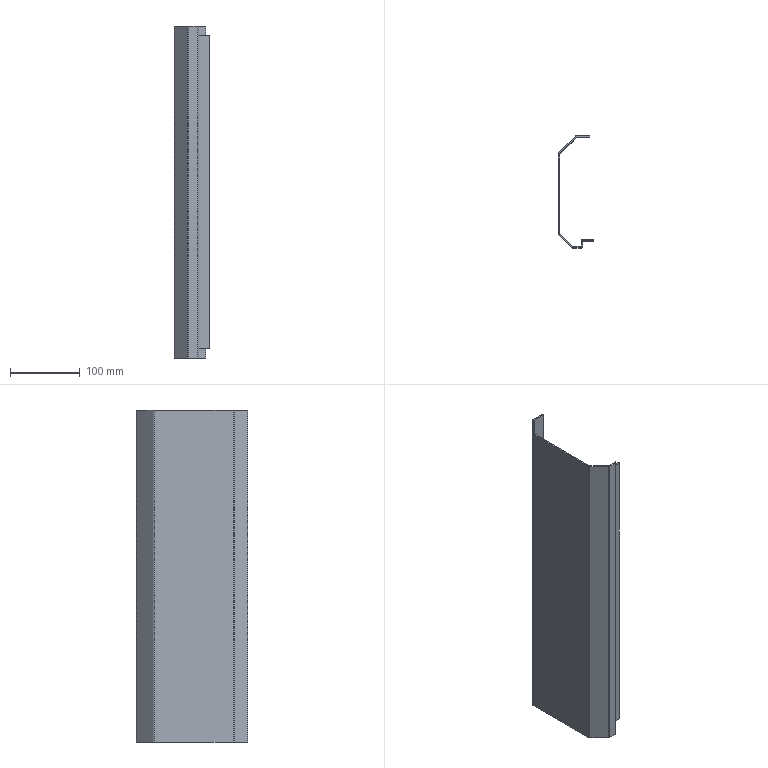Part | STEP file | Control Box 1 | 1 solid | 34 faces | box 51 x 160 x 476 mm | volume 222530 mm3 | plane 22 | cylinder 12 | commonest cylinder face diameters 0.2 x6 4.2 x6
STEP:
#1=CARTESIAN_POINT('',(-54.818,-25.87,476.));
#2=VERTEX_POINT('',#1);
#3=CARTESIAN_POINT('',(-54.818,-139.13,476.));
#4=VERTEX_POINT('',#3);
#5=CARTESIAN_POINT('',(-54.818,-25.,476.));
#6=DIRECTION('',(0.,-1.,0.));
#7=VECTOR('',#6,1000.);
#8=LINE('',#5,#7);
#9=EDGE_CURVE('',#2,#4,#8,.T.);
#10=ORIENTED_EDGE('',*,*,#9,.T.);
#11=CARTESIAN_POINT('',(-54.818,-139.13,0.));
#12=VERTEX_POINT('',#11);
#13=CARTESIAN_POINT('',(-54.818,-139.13,476.));
#14=DIRECTION('',(0.,0.,-1.));
#15=VECTOR('',#14,1000.);
#16=LINE('',#13,#15);
#17=EDGE_CURVE('',#4,#12,#16,.T.);
#18=ORIENTED_EDGE('',*,*,#17,.T.);
#19=CARTESIAN_POINT('',(-54.818,-25.87,0.));
#20=VERTEX_POINT('',#19);
#21=CARTESIAN_POINT('',(-54.818,-25.,0.));
#22=DIRECTION('',(0.,1.,0.));
#23=VECTOR('',#22,1000.);
#24=LINE('',#21,#23);
#25=EDGE_CURVE('',#12,#20,#24,.T.);
#26=ORIENTED_EDGE('',*,*,#25,.T.);
#27=CARTESIAN_POINT('',(-54.818,-25.87,476.));
#28=DIRECTION('',(0.,0.,1.));
#29=VECTOR('',#28,1000.);
#30=LINE('',#27,#29);
#31=EDGE_CURVE('',#20,#2,#30,.T.);
#32=ORIENTED_EDGE('',*,*,#31,.T.);
#33=EDGE_LOOP('',(#10,#18,#26,#32));
#34=FACE_OUTER_BOUND('',#33,.T.);
#35=CARTESIAN_POINT('',(-54.818,-25.,476.));
#36=DIRECTION('',(1.,0.,0.));
#37=DIRECTION('',(0.,1.,0.));
#38=AXIS2_PLACEMENT_3D('',#35,#36,#37);
#39=PLANE('',#38);
#40=ADVANCED_FACE('',(#34),#39,.T.);
#41=ORIENTED_EDGE('',*,*,#17,.F.);
#42=CARTESIAN_POINT('',(-54.789,-139.201,476.));
#43=VERTEX_POINT('',#42);
#44=CARTESIAN_POINT('',(-54.718,-139.13,476.));
#45=DIRECTION('',(0.,0.,-1.));
#46=DIRECTION('',(-1.,0.,0.));
#47=AXIS2_PLACEMENT_3D('',#44,#45,#46);
#48=CIRCLE('',#47,0.1);
#49=EDGE_CURVE('',#43,#4,#48,.T.);
#50=ORIENTED_EDGE('',*,*,#49,.F.);
#51=CARTESIAN_POINT('',(-54.789,-139.201,0.));
#52=VERTEX_POINT('',#51);
#53=CARTESIAN_POINT('',(-54.789,-139.201,476.));
#54=DIRECTION('',(0.,0.,1.));
#55=VECTOR('',#54,1000.);
#56=LINE('',#53,#55);
#57=EDGE_CURVE('',#52,#43,#56,.T.);
#58=ORIENTED_EDGE('',*,*,#57,.F.);
#59=CARTESIAN_POINT('',(-54.718,-139.13,0.));
#60=DIRECTION('',(0.,0.,1.));
#61=DIRECTION('',(-1.,0.,0.));
#62=AXIS2_PLACEMENT_3D('',#59,#60,#61);
#63=CIRCLE('',#62,0.1);
#64=EDGE_CURVE('',#12,#52,#63,.T.);
#65=ORIENTED_EDGE('',*,*,#64,.F.);
#66=EDGE_LOOP('',(#41,#50,#58,#65));
#67=FACE_OUTER_BOUND('',#66,.T.);
#68=CARTESIAN_POINT('',(-54.718,-139.13,476.));
#69=DIRECTION('',(0.,0.,-1.));
#70=DIRECTION('',(-1.,0.,0.));
#71=AXIS2_PLACEMENT_3D('',#68,#69,#70);
#72=CYLINDRICAL_SURFACE('',#71,0.1);
#73=ADVANCED_FACE('',(#67),#72,.F.);
#74=ORIENTED_EDGE('',*,*,#9,.F.);
#75=CARTESIAN_POINT('',(-54.789,-25.799,476.));
#76=VERTEX_POINT('',#75);
#77=CARTESIAN_POINT('',(-54.718,-25.87,476.));
#78=DIRECTION('',(0.,0.,-1.));
#79=DIRECTION('',(-1.,0.,0.));
#80=AXIS2_PLACEMENT_3D('',#77,#78,#79);
#81=CIRCLE('',#80,0.1);
#82=EDGE_CURVE('',#2,#76,#81,.T.);
#83=ORIENTED_EDGE('',*,*,#82,.T.);
#84=CARTESIAN_POINT('',(-31.019,-2.029,476.));
#85=VERTEX_POINT('',#84);
#86=CARTESIAN_POINT('',(-30.404,-1.414,476.));
#87=DIRECTION('',(-0.7071,-0.7071,0.));
#88=VECTOR('',#87,1000.);
#89=LINE('',#86,#88);
#90=EDGE_CURVE('',#85,#76,#89,.T.);
#91=ORIENTED_EDGE('',*,*,#90,.F.);
#92=CARTESIAN_POINT('',(-30.948,-2.,476.));
#93=VERTEX_POINT('',#92);
#94=CARTESIAN_POINT('',(-30.948,-2.1,476.));
#95=DIRECTION('',(0.,0.,-1.));
#96=DIRECTION('',(-1.,0.,0.));
#97=AXIS2_PLACEMENT_3D('',#94,#95,#96);
#98=CIRCLE('',#97,0.1);
#99=EDGE_CURVE('',#85,#93,#98,.T.);
#100=ORIENTED_EDGE('',*,*,#99,.T.);
#101=CARTESIAN_POINT('',(-11.818,-2.,476.));
#102=VERTEX_POINT('',#101);
#103=CARTESIAN_POINT('',(-31.818,-2.,476.));
#104=DIRECTION('',(-1.,0.,0.));
#105=VECTOR('',#104,1000.);
#106=LINE('',#103,#105);
#107=EDGE_CURVE('',#102,#93,#106,.T.);
#108=ORIENTED_EDGE('',*,*,#107,.F.);
#109=CARTESIAN_POINT('',(-11.818,0.,476.));
#110=VERTEX_POINT('',#109);
#111=CARTESIAN_POINT('',(-11.818,-2.029,476.));
#112=DIRECTION('',(0.,1.,0.));
#113=VECTOR('',#112,1000.);
#114=LINE('',#111,#113);
#115=EDGE_CURVE('',#102,#110,#114,.T.);
#116=ORIENTED_EDGE('',*,*,#115,.T.);
#117=CARTESIAN_POINT('',(-30.948,0.,476.));
#118=VERTEX_POINT('',#117);
#119=CARTESIAN_POINT('',(-31.019,0.,476.));
#120=DIRECTION('',(-1.,0.,0.));
#121=VECTOR('',#120,1000.);
#122=LINE('',#119,#121);
#123=EDGE_CURVE('',#110,#118,#122,.T.);
#124=ORIENTED_EDGE('',*,*,#123,.T.);
#125=CARTESIAN_POINT('',(-32.433,-0.6151,476.));
#126=VERTEX_POINT('',#125);
#127=CARTESIAN_POINT('',(-30.948,-2.1,476.));
#128=DIRECTION('',(0.,0.,-1.));
#129=DIRECTION('',(-1.,0.,0.));
#130=AXIS2_PLACEMENT_3D('',#127,#128,#129);
#131=CIRCLE('',#130,2.1);
#132=EDGE_CURVE('',#126,#118,#131,.T.);
#133=ORIENTED_EDGE('',*,*,#132,.F.);
#134=CARTESIAN_POINT('',(-56.203,-24.385,476.));
#135=VERTEX_POINT('',#134);
#136=CARTESIAN_POINT('',(-32.433,-0.6151,476.));
#137=DIRECTION('',(-0.7071,-0.7071,0.));
#138=VECTOR('',#137,1000.);
#139=LINE('',#136,#138);
#140=EDGE_CURVE('',#126,#135,#139,.T.);
#141=ORIENTED_EDGE('',*,*,#140,.T.);
#142=CARTESIAN_POINT('',(-56.818,-25.87,476.));
#143=VERTEX_POINT('',#142);
#144=CARTESIAN_POINT('',(-54.718,-25.87,476.));
#145=DIRECTION('',(0.,0.,-1.));
#146=DIRECTION('',(-1.,0.,0.));
#147=AXIS2_PLACEMENT_3D('',#144,#145,#146);
#148=CIRCLE('',#147,2.1);
#149=EDGE_CURVE('',#143,#135,#148,.T.);
#150=ORIENTED_EDGE('',*,*,#149,.F.);
#151=CARTESIAN_POINT('',(-56.818,-139.13,476.));
#152=VERTEX_POINT('',#151);
#153=CARTESIAN_POINT('',(-56.818,-139.201,476.));
#154=DIRECTION('',(0.,-1.,0.));
#155=VECTOR('',#154,1000.);
#156=LINE('',#153,#155);
#157=EDGE_CURVE('',#143,#152,#156,.T.);
#158=ORIENTED_EDGE('',*,*,#157,.T.);
#159=CARTESIAN_POINT('',(-56.203,-140.615,476.));
#160=VERTEX_POINT('',#159);
#161=CARTESIAN_POINT('',(-54.718,-139.13,476.));
#162=DIRECTION('',(0.,0.,-1.));
#163=DIRECTION('',(-1.,0.,0.));
#164=AXIS2_PLACEMENT_3D('',#161,#162,#163);
#165=CIRCLE('',#164,2.1);
#166=EDGE_CURVE('',#160,#152,#165,.T.);
#167=ORIENTED_EDGE('',*,*,#166,.F.);
#168=CARTESIAN_POINT('',(-37.433,-159.385,476.));
#169=VERTEX_POINT('',#168);
#170=CARTESIAN_POINT('',(-56.203,-140.615,476.));
#171=DIRECTION('',(0.7071,-0.7071,0.));
#172=VECTOR('',#171,1000.);
#173=LINE('',#170,#172);
#174=EDGE_CURVE('',#160,#169,#173,.T.);
#175=ORIENTED_EDGE('',*,*,#174,.T.);
#176=CARTESIAN_POINT('',(-35.948,-160.,476.));
#177=VERTEX_POINT('',#176);
#178=CARTESIAN_POINT('',(-35.948,-157.9,476.));
#179=DIRECTION('',(0.,0.,-1.));
#180=DIRECTION('',(-1.,0.,0.));
#181=AXIS2_PLACEMENT_3D('',#178,#179,#180);
#182=CIRCLE('',#181,2.1);
#183=EDGE_CURVE('',#177,#169,#182,.T.);
#184=ORIENTED_EDGE('',*,*,#183,.F.);
#185=CARTESIAN_POINT('',(-23.918,-160.,476.));
#186=VERTEX_POINT('',#185);
#187=CARTESIAN_POINT('',(-35.948,-160.,476.));
#188=DIRECTION('',(1.,0.,0.));
#189=VECTOR('',#188,1000.);
#190=LINE('',#187,#189);
#191=EDGE_CURVE('',#177,#186,#190,.T.);
#192=ORIENTED_EDGE('',*,*,#191,.T.);
#193=CARTESIAN_POINT('',(-21.818,-157.9,476.));
#194=VERTEX_POINT('',#193);
#195=CARTESIAN_POINT('',(-23.918,-157.9,476.));
#196=DIRECTION('',(0.,0.,1.));
#197=DIRECTION('',(-1.,0.,0.));
#198=AXIS2_PLACEMENT_3D('',#195,#196,#197);
#199=CIRCLE('',#198,2.1);
#200=EDGE_CURVE('',#186,#194,#199,.T.);
#201=ORIENTED_EDGE('',*,*,#200,.T.);
#202=CARTESIAN_POINT('',(-23.818,-157.9,476.));
#203=VERTEX_POINT('',#202);
#204=CARTESIAN_POINT('',(-21.818,-157.9,476.));
#205=DIRECTION('',(-1.,0.,0.));
#206=VECTOR('',#205,1000.);
#207=LINE('',#204,#206);
#208=EDGE_CURVE('',#194,#203,#207,.T.);
#209=ORIENTED_EDGE('',*,*,#208,.T.);
#210=CARTESIAN_POINT('',(-23.918,-158.,476.));
#211=VERTEX_POINT('',#210);
#212=CARTESIAN_POINT('',(-23.918,-157.9,476.));
#213=DIRECTION('',(0.,0.,-1.));
#214=DIRECTION('',(-1.,0.,0.));
#215=AXIS2_PLACEMENT_3D('',#212,#213,#214);
#216=CIRCLE('',#215,0.1);
#217=EDGE_CURVE('',#203,#211,#216,.T.);
#218=ORIENTED_EDGE('',*,*,#217,.T.);
#219=CARTESIAN_POINT('',(-35.948,-158.,476.));
#220=VERTEX_POINT('',#219);
#221=CARTESIAN_POINT('',(-36.818,-158.,476.));
#222=DIRECTION('',(1.,0.,0.));
#223=VECTOR('',#222,1000.);
#224=LINE('',#221,#223);
#225=EDGE_CURVE('',#220,#211,#224,.T.);
#226=ORIENTED_EDGE('',*,*,#225,.F.);
#227=CARTESIAN_POINT('',(-36.019,-157.971,476.));
#228=VERTEX_POINT('',#227);
#229=CARTESIAN_POINT('',(-35.948,-157.9,476.));
#230=DIRECTION('',(0.,0.,-1.));
#231=DIRECTION('',(-1.,0.,0.));
#232=AXIS2_PLACEMENT_3D('',#229,#230,#231);
#233=CIRCLE('',#232,0.1);
#234=EDGE_CURVE('',#220,#228,#233,.T.);
#235=ORIENTED_EDGE('',*,*,#234,.T.);
#236=CARTESIAN_POINT('',(-55.404,-138.586,476.));
#237=DIRECTION('',(0.7071,-0.7071,0.));
#238=VECTOR('',#237,1000.);
#239=LINE('',#236,#238);
#240=EDGE_CURVE('',#43,#228,#239,.T.);
#241=ORIENTED_EDGE('',*,*,#240,.F.);
#242=ORIENTED_EDGE('',*,*,#49,.T.);
#243=EDGE_LOOP('',(#74,#83,#91,#100,#108,#116,#124,#133,#141,#150,#158,#167,#175,#184,#192,#201,#209,#218,#226,#235,#241,#242));
#244=FACE_OUTER_BOUND('',#243,.T.);
#245=CARTESIAN_POINT('',(-54.789,-139.201,476.));
#246=DIRECTION('',(0.,0.,1.));
#247=DIRECTION('',(1.,0.,0.));
#248=AXIS2_PLACEMENT_3D('',#245,#246,#247);
#249=PLANE('',#248);
#250=ADVANCED_FACE('',(#244),#249,.T.);
#251=CARTESIAN_POINT('',(-54.789,-25.799,0.));
#252=VERTEX_POINT('',#251);
#253=CARTESIAN_POINT('',(-54.789,-25.799,476.));
#254=DIRECTION('',(0.,0.,-1.));
#255=VECTOR('',#254,1000.);
#256=LINE('',#253,#255);
#257=EDGE_CURVE('',#76,#252,#256,.T.);
#258=ORIENTED_EDGE('',*,*,#257,.F.);
#259=ORIENTED_EDGE('',*,*,#82,.F.);
#260=ORIENTED_EDGE('',*,*,#31,.F.);
#261=CARTESIAN_POINT('',(-54.718,-25.87,0.));
#262=DIRECTION('',(0.,0.,1.));
#263=DIRECTION('',(-1.,0.,0.));
#264=AXIS2_PLACEMENT_3D('',#261,#262,#263);
#265=CIRCLE('',#264,0.1);
#266=EDGE_CURVE('',#252,#20,#265,.T.);
#267=ORIENTED_EDGE('',*,*,#266,.F.);
#268=EDGE_LOOP('',(#258,#259,#260,#267));
#269=FACE_OUTER_BOUND('',#268,.T.);
#270=CARTESIAN_POINT('',(-54.718,-25.87,476.));
#271=DIRECTION('',(0.,0.,-1.));
#272=DIRECTION('',(-1.,0.,0.));
#273=AXIS2_PLACEMENT_3D('',#270,#271,#272);
#274=CYLINDRICAL_SURFACE('',#273,0.1);
#275=ADVANCED_FACE('',(#269),#274,.F.);
#276=ORIENTED_EDGE('',*,*,#25,.F.);
#277=ORIENTED_EDGE('',*,*,#64,.T.);
#278=CARTESIAN_POINT('',(-36.019,-157.971,0.));
#279=VERTEX_POINT('',#278);
#280=CARTESIAN_POINT('',(-55.404,-138.586,0.));
#281=DIRECTION('',(-0.7071,0.7071,0.));
#282=VECTOR('',#281,1000.);
#283=LINE('',#280,#282);
#284=EDGE_CURVE('',#279,#52,#283,.T.);
#285=ORIENTED_EDGE('',*,*,#284,.F.);
#286=CARTESIAN_POINT('',(-35.948,-158.,0.));
#287=VERTEX_POINT('',#286);
#288=CARTESIAN_POINT('',(-35.948,-157.9,0.));
#289=DIRECTION('',(0.,0.,1.));
#290=DIRECTION('',(-1.,0.,0.));
#291=AXIS2_PLACEMENT_3D('',#288,#289,#290);
#292=CIRCLE('',#291,0.1);
#293=EDGE_CURVE('',#279,#287,#292,.T.);
#294=ORIENTED_EDGE('',*,*,#293,.T.);
#295=CARTESIAN_POINT('',(-23.918,-158.,0.));
#296=VERTEX_POINT('',#295);
#297=CARTESIAN_POINT('',(-36.818,-158.,0.));
#298=DIRECTION('',(-1.,0.,0.));
#299=VECTOR('',#298,1000.);
#300=LINE('',#297,#299);
#301=EDGE_CURVE('',#296,#287,#300,.T.);
#302=ORIENTED_EDGE('',*,*,#301,.F.);
#303=CARTESIAN_POINT('',(-23.818,-157.9,0.));
#304=VERTEX_POINT('',#303);
#305=CARTESIAN_POINT('',(-23.918,-157.9,0.));
#306=DIRECTION('',(0.,0.,1.));
#307=DIRECTION('',(-1.,0.,0.));
#308=AXIS2_PLACEMENT_3D('',#305,#306,#307);
#309=CIRCLE('',#308,0.1);
#310=EDGE_CURVE('',#296,#304,#309,.T.);
#311=ORIENTED_EDGE('',*,*,#310,.T.);
#312=CARTESIAN_POINT('',(-21.818,-157.9,0.));
#313=VERTEX_POINT('',#312);
#314=CARTESIAN_POINT('',(-23.918,-157.9,0.));
#315=DIRECTION('',(-1.,0.,0.));
#316=VECTOR('',#315,1000.);
#317=LINE('',#314,#316);
#318=EDGE_CURVE('',#313,#304,#317,.T.);
#319=ORIENTED_EDGE('',*,*,#318,.F.);
#320=CARTESIAN_POINT('',(-23.918,-160.,0.));
#321=VERTEX_POINT('',#320);
#322=CARTESIAN_POINT('',(-23.918,-157.9,0.));
#323=DIRECTION('',(0.,0.,1.));
#324=DIRECTION('',(-1.,0.,0.));
#325=AXIS2_PLACEMENT_3D('',#322,#323,#324);
#326=CIRCLE('',#325,2.1);
#327=EDGE_CURVE('',#321,#313,#326,.T.);
#328=ORIENTED_EDGE('',*,*,#327,.F.);
#329=CARTESIAN_POINT('',(-35.948,-160.,0.));
#330=VERTEX_POINT('',#329);
#331=CARTESIAN_POINT('',(-36.019,-160.,0.));
#332=DIRECTION('',(-1.,0.,0.));
#333=VECTOR('',#332,1000.);
#334=LINE('',#331,#333);
#335=EDGE_CURVE('',#321,#330,#334,.T.);
#336=ORIENTED_EDGE('',*,*,#335,.T.);
#337=CARTESIAN_POINT('',(-37.433,-159.385,0.));
#338=VERTEX_POINT('',#337);
#339=CARTESIAN_POINT('',(-35.948,-157.9,0.));
#340=DIRECTION('',(0.,0.,-1.));
#341=DIRECTION('',(-1.,0.,0.));
#342=AXIS2_PLACEMENT_3D('',#339,#340,#341);
#343=CIRCLE('',#342,2.1);
#344=EDGE_CURVE('',#330,#338,#343,.T.);
#345=ORIENTED_EDGE('',*,*,#344,.T.);
#346=CARTESIAN_POINT('',(-56.203,-140.615,0.));
#347=VERTEX_POINT('',#346);
#348=CARTESIAN_POINT('',(-37.433,-159.385,0.));
#349=DIRECTION('',(-0.7071,0.7071,0.));
#350=VECTOR('',#349,1000.);
#351=LINE('',#348,#350);
#352=EDGE_CURVE('',#338,#347,#351,.T.);
#353=ORIENTED_EDGE('',*,*,#352,.T.);
#354=CARTESIAN_POINT('',(-56.818,-139.13,0.));
#355=VERTEX_POINT('',#354);
#356=CARTESIAN_POINT('',(-54.718,-139.13,0.));
#357=DIRECTION('',(0.,0.,-1.));
#358=DIRECTION('',(-1.,0.,0.));
#359=AXIS2_PLACEMENT_3D('',#356,#357,#358);
#360=CIRCLE('',#359,2.1);
#361=EDGE_CURVE('',#347,#355,#360,.T.);
#362=ORIENTED_EDGE('',*,*,#361,.T.);
#363=CARTESIAN_POINT('',(-56.818,-25.87,0.));
#364=VERTEX_POINT('',#363);
#365=CARTESIAN_POINT('',(-56.818,-25.799,0.));
#366=DIRECTION('',(0.,1.,0.));
#367=VECTOR('',#366,1000.);
#368=LINE('',#365,#367);
#369=EDGE_CURVE('',#355,#364,#368,.T.);
#370=ORIENTED_EDGE('',*,*,#369,.T.);
#371=CARTESIAN_POINT('',(-56.203,-24.385,0.));
#372=VERTEX_POINT('',#371);
#373=CARTESIAN_POINT('',(-54.718,-25.87,0.));
#374=DIRECTION('',(0.,0.,-1.));
#375=DIRECTION('',(-1.,0.,0.));
#376=AXIS2_PLACEMENT_3D('',#373,#374,#375);
#377=CIRCLE('',#376,2.1);
#378=EDGE_CURVE('',#364,#372,#377,.T.);
#379=ORIENTED_EDGE('',*,*,#378,.T.);
#380=CARTESIAN_POINT('',(-32.433,-0.6151,0.));
#381=VERTEX_POINT('',#380);
#382=CARTESIAN_POINT('',(-56.203,-24.385,0.));
#383=DIRECTION('',(0.7071,0.7071,0.));
#384=VECTOR('',#383,1000.);
#385=LINE('',#382,#384);
#386=EDGE_CURVE('',#372,#381,#385,.T.);
#387=ORIENTED_EDGE('',*,*,#386,.T.);
#388=CARTESIAN_POINT('',(-30.948,0.,0.));
#389=VERTEX_POINT('',#388);
#390=CARTESIAN_POINT('',(-30.948,-2.1,0.));
#391=DIRECTION('',(0.,0.,-1.));
#392=DIRECTION('',(-1.,0.,0.));
#393=AXIS2_PLACEMENT_3D('',#390,#391,#392);
#394=CIRCLE('',#393,2.1);
#395=EDGE_CURVE('',#381,#389,#394,.T.);
#396=ORIENTED_EDGE('',*,*,#395,.T.);
#397=CARTESIAN_POINT('',(-11.818,0.,0.));
#398=VERTEX_POINT('',#397);
#399=CARTESIAN_POINT('',(-35.948,0.,0.));
#400=DIRECTION('',(-1.,0.,0.));
#401=VECTOR('',#400,1000.);
#402=LINE('',#399,#401);
#403=EDGE_CURVE('',#398,#389,#402,.T.);
#404=ORIENTED_EDGE('',*,*,#403,.F.);
#405=CARTESIAN_POINT('',(-11.818,-2.,0.));
#406=VERTEX_POINT('',#405);
#407=CARTESIAN_POINT('',(-11.818,0.,0.));
#408=DIRECTION('',(0.,1.,0.));
#409=VECTOR('',#408,1000.);
#410=LINE('',#407,#409);
#411=EDGE_CURVE('',#406,#398,#410,.T.);
#412=ORIENTED_EDGE('',*,*,#411,.F.);
#413=CARTESIAN_POINT('',(-30.948,-2.,0.));
#414=VERTEX_POINT('',#413);
#415=CARTESIAN_POINT('',(-31.818,-2.,0.));
#416=DIRECTION('',(1.,0.,0.));
#417=VECTOR('',#416,1000.);
#418=LINE('',#415,#417);
#419=EDGE_CURVE('',#414,#406,#418,.T.);
#420=ORIENTED_EDGE('',*,*,#419,.F.);
#421=CARTESIAN_POINT('',(-31.019,-2.029,0.));
#422=VERTEX_POINT('',#421);
#423=CARTESIAN_POINT('',(-30.948,-2.1,0.));
#424=DIRECTION('',(0.,0.,1.));
#425=DIRECTION('',(-1.,0.,0.));
#426=AXIS2_PLACEMENT_3D('',#423,#424,#425);
#427=CIRCLE('',#426,0.1);
#428=EDGE_CURVE('',#414,#422,#427,.T.);
#429=ORIENTED_EDGE('',*,*,#428,.T.);
#430=CARTESIAN_POINT('',(-30.404,-1.414,0.));
#431=DIRECTION('',(0.7071,0.7071,0.));
#432=VECTOR('',#431,1000.);
#433=LINE('',#430,#432);
#434=EDGE_CURVE('',#252,#422,#433,.T.);
#435=ORIENTED_EDGE('',*,*,#434,.F.);
#436=ORIENTED_EDGE('',*,*,#266,.T.);
#437=EDGE_LOOP('',(#276,#277,#285,#294,#302,#311,#319,#328,#336,#345,#353,#362,#370,#379,#387,#396,#404,#412,#420,#429,#435,#436));
#438=FACE_OUTER_BOUND('',#437,.T.);
#439=CARTESIAN_POINT('',(-54.789,-25.799,0.));
#440=DIRECTION('',(0.,0.,-1.));
#441=DIRECTION('',(-1.,0.,0.));
#442=AXIS2_PLACEMENT_3D('',#439,#440,#441);
#443=PLANE('',#442);
#444=ADVANCED_FACE('',(#438),#443,.T.);
#445=ORIENTED_EDGE('',*,*,#240,.T.);
#446=CARTESIAN_POINT('',(-36.019,-157.971,476.));
#447=DIRECTION('',(0.,0.,-1.));
#448=VECTOR('',#447,1000.);
#449=LINE('',#446,#448);
#450=EDGE_CURVE('',#228,#279,#449,.T.);
#451=ORIENTED_EDGE('',*,*,#450,.T.);
#452=ORIENTED_EDGE('',*,*,#284,.T.);
#453=ORIENTED_EDGE('',*,*,#57,.T.);
#454=EDGE_LOOP('',(#445,#451,#452,#453));
#455=FACE_OUTER_BOUND('',#454,.T.);
#456=CARTESIAN_POINT('',(-55.404,-138.586,476.));
#457=DIRECTION('',(0.7071,0.7071,0.));
#458=DIRECTION('',(-0.7071,0.7071,0.));
#459=AXIS2_PLACEMENT_3D('',#456,#457,#458);
#460=PLANE('',#459);
#461=ADVANCED_FACE('',(#455),#460,.T.);
#462=CARTESIAN_POINT('',(-56.818,-139.13,476.));
#463=DIRECTION('',(0.,0.,-1.));
#464=VECTOR('',#463,1000.);
#465=LINE('',#462,#464);
#466=EDGE_CURVE('',#152,#355,#465,.T.);
#467=ORIENTED_EDGE('',*,*,#466,.F.);
#468=ORIENTED_EDGE('',*,*,#157,.F.);
#469=CARTESIAN_POINT('',(-56.818,-25.87,476.));
#470=DIRECTION('',(0.,0.,1.));
#471=VECTOR('',#470,1000.);
#472=LINE('',#469,#471);
#473=EDGE_CURVE('',#364,#143,#472,.T.);
#474=ORIENTED_EDGE('',*,*,#473,.F.);
#475=ORIENTED_EDGE('',*,*,#369,.F.);
#476=EDGE_LOOP('',(#467,#468,#474,#475));
#477=FACE_OUTER_BOUND('',#476,.T.);
#478=CARTESIAN_POINT('',(-56.818,-25.,476.));
#479=DIRECTION('',(1.,0.,0.));
#480=DIRECTION('',(0.,1.,0.));
#481=AXIS2_PLACEMENT_3D('',#478,#479,#480);
#482=PLANE('',#481);
#483=ADVANCED_FACE('',(#477),#482,.F.);
#484=ORIENTED_EDGE('',*,*,#90,.T.);
#485=ORIENTED_EDGE('',*,*,#257,.T.);
#486=ORIENTED_EDGE('',*,*,#434,.T.);
#487=CARTESIAN_POINT('',(-31.019,-2.029,476.));
#488=DIRECTION('',(0.,0.,1.));
#489=VECTOR('',#488,1000.);
#490=LINE('',#487,#489);
#491=EDGE_CURVE('',#422,#85,#490,.T.);
#492=ORIENTED_EDGE('',*,*,#491,.T.);
#493=EDGE_LOOP('',(#484,#485,#486,#492));
#494=FACE_OUTER_BOUND('',#493,.T.);
#495=CARTESIAN_POINT('',(-30.404,-1.414,476.));
#496=DIRECTION('',(0.7071,-0.7071,0.));
#497=DIRECTION('',(0.7071,0.7071,0.));
#498=AXIS2_PLACEMENT_3D('',#495,#496,#497);
#499=PLANE('',#498);
#500=ADVANCED_FACE('',(#494),#499,.T.);
#501=ORIENTED_EDGE('',*,*,#450,.F.);
#502=ORIENTED_EDGE('',*,*,#234,.F.);
#503=CARTESIAN_POINT('',(-35.948,-158.,476.));
#504=DIRECTION('',(0.,0.,1.));
#505=VECTOR('',#504,1000.);
#506=LINE('',#503,#505);
#507=EDGE_CURVE('',#287,#220,#506,.T.);
#508=ORIENTED_EDGE('',*,*,#507,.F.);
#509=ORIENTED_EDGE('',*,*,#293,.F.);
#510=EDGE_LOOP('',(#501,#502,#508,#509));
#511=FACE_OUTER_BOUND('',#510,.T.);
#512=CARTESIAN_POINT('',(-35.948,-157.9,476.));
#513=DIRECTION('',(0.,0.,-1.));
#514=DIRECTION('',(-1.,0.,0.));
#515=AXIS2_PLACEMENT_3D('',#512,#513,#514);
#516=CYLINDRICAL_SURFACE('',#515,0.1);
#517=ADVANCED_FACE('',(#511),#516,.F.);
#518=ORIENTED_EDGE('',*,*,#166,.T.);
#519=ORIENTED_EDGE('',*,*,#466,.T.);
#520=ORIENTED_EDGE('',*,*,#361,.F.);
#521=CARTESIAN_POINT('',(-56.203,-140.615,476.));
#522=DIRECTION('',(0.,0.,1.));
#523=VECTOR('',#522,1000.);
#524=LINE('',#521,#523);
#525=EDGE_CURVE('',#347,#160,#524,.T.);
#526=ORIENTED_EDGE('',*,*,#525,.T.);
#527=EDGE_LOOP('',(#518,#519,#520,#526));
#528=FACE_OUTER_BOUND('',#527,.T.);
#529=CARTESIAN_POINT('',(-54.718,-139.13,476.));
#530=DIRECTION('',(0.,0.,-1.));
#531=DIRECTION('',(-1.,0.,0.));
#532=AXIS2_PLACEMENT_3D('',#529,#530,#531);
#533=CYLINDRICAL_SURFACE('',#532,2.1);
#534=ADVANCED_FACE('',(#528),#533,.T.);
#535=ORIENTED_EDGE('',*,*,#149,.T.);
#536=CARTESIAN_POINT('',(-56.203,-24.385,476.));
#537=DIRECTION('',(0.,0.,-1.));
#538=VECTOR('',#537,1000.);
#539=LINE('',#536,#538);
#540=EDGE_CURVE('',#135,#372,#539,.T.);
#541=ORIENTED_EDGE('',*,*,#540,.T.);
#542=ORIENTED_EDGE('',*,*,#378,.F.);
#543=ORIENTED_EDGE('',*,*,#473,.T.);
#544=EDGE_LOOP('',(#535,#541,#542,#543));
#545=FACE_OUTER_BOUND('',#544,.T.);
#546=CARTESIAN_POINT('',(-54.718,-25.87,476.));
#547=DIRECTION('',(0.,0.,-1.));
#548=DIRECTION('',(-1.,0.,0.));
#549=AXIS2_PLACEMENT_3D('',#546,#547,#548);
#550=CYLINDRICAL_SURFACE('',#549,2.1);
#551=ADVANCED_FACE('',(#545),#550,.T.);
#552=CARTESIAN_POINT('',(-30.948,-2.,476.));
#553=DIRECTION('',(0.,0.,-1.));
#554=VECTOR('',#553,1000.);
#555=LINE('',#552,#554);
#556=EDGE_CURVE('',#93,#414,#555,.T.);
#557=ORIENTED_EDGE('',*,*,#556,.F.);
#558=ORIENTED_EDGE('',*,*,#99,.F.);
#559=ORIENTED_EDGE('',*,*,#491,.F.);
#560=ORIENTED_EDGE('',*,*,#428,.F.);
#561=EDGE_LOOP('',(#557,#558,#559,#560));
#562=FACE_OUTER_BOUND('',#561,.T.);
#563=CARTESIAN_POINT('',(-30.948,-2.1,476.));
#564=DIRECTION('',(0.,0.,-1.));
#565=DIRECTION('',(-1.,0.,0.));
#566=AXIS2_PLACEMENT_3D('',#563,#564,#565);
#567=CYLINDRICAL_SURFACE('',#566,0.1);
#568=ADVANCED_FACE('',(#562),#567,.F.);
#569=ORIENTED_EDGE('',*,*,#301,.T.);
#570=ORIENTED_EDGE('',*,*,#507,.T.);
#571=ORIENTED_EDGE('',*,*,#225,.T.);
#572=CARTESIAN_POINT('',(-23.918,-158.,476.));
#573=DIRECTION('',(0.,0.,-1.));
#574=VECTOR('',#573,1000.);
#575=LINE('',#572,#574);
#576=EDGE_CURVE('',#211,#296,#575,.T.);
#577=ORIENTED_EDGE('',*,*,#576,.T.);
#578=EDGE_LOOP('',(#569,#570,#571,#577));
#579=FACE_OUTER_BOUND('',#578,.T.);
#580=CARTESIAN_POINT('',(-36.818,-158.,476.));
#581=DIRECTION('',(0.,1.,0.));
#582=DIRECTION('',(0.,0.,1.));
#583=AXIS2_PLACEMENT_3D('',#580,#581,#582);
#584=PLANE('',#583);
#585=ADVANCED_FACE('',(#579),#584,.T.);
#586=CARTESIAN_POINT('',(-37.433,-159.385,476.));
#587=DIRECTION('',(0.,0.,-1.));
#588=VECTOR('',#587,1000.);
#589=LINE('',#586,#588);
#590=EDGE_CURVE('',#169,#338,#589,.T.);
#591=ORIENTED_EDGE('',*,*,#590,.F.);
#592=ORIENTED_EDGE('',*,*,#174,.F.);
#593=ORIENTED_EDGE('',*,*,#525,.F.);
#594=ORIENTED_EDGE('',*,*,#352,.F.);
#595=EDGE_LOOP('',(#591,#592,#593,#594));
#596=FACE_OUTER_BOUND('',#595,.T.);
#597=CARTESIAN_POINT('',(-56.818,-140.,476.));
#598=DIRECTION('',(0.7071,0.7071,0.));
#599=DIRECTION('',(-0.7071,0.7071,0.));
#600=AXIS2_PLACEMENT_3D('',#597,#598,#599);
#601=PLANE('',#600);
#602=ADVANCED_FACE('',(#596),#601,.F.);
#603=ORIENTED_EDGE('',*,*,#540,.F.);
#604=ORIENTED_EDGE('',*,*,#140,.F.);
#605=CARTESIAN_POINT('',(-32.433,-0.6151,476.));
#606=DIRECTION('',(0.,0.,1.));
#607=VECTOR('',#606,1000.);
#608=LINE('',#605,#607);
#609=EDGE_CURVE('',#381,#126,#608,.T.);
#610=ORIENTED_EDGE('',*,*,#609,.F.);
#611=ORIENTED_EDGE('',*,*,#386,.F.);
#612=EDGE_LOOP('',(#603,#604,#610,#611));
#613=FACE_OUTER_BOUND('',#612,.T.);
#614=CARTESIAN_POINT('',(-31.818,0.,476.));
#615=DIRECTION('',(0.7071,-0.7071,0.));
#616=DIRECTION('',(0.7071,0.7071,0.));
#617=AXIS2_PLACEMENT_3D('',#614,#615,#616);
#618=PLANE('',#617);
#619=ADVANCED_FACE('',(#613),#618,.F.);
#620=ORIENTED_EDGE('',*,*,#107,.T.);
#621=ORIENTED_EDGE('',*,*,#556,.T.);
#622=ORIENTED_EDGE('',*,*,#419,.T.);
#623=CARTESIAN_POINT('',(-11.818,-2.,476.));
#624=DIRECTION('',(0.,0.,1.));
#625=VECTOR('',#624,1000.);
#626=LINE('',#623,#625);
#627=EDGE_CURVE('',#406,#102,#626,.T.);
#628=ORIENTED_EDGE('',*,*,#627,.T.);
#629=EDGE_LOOP('',(#620,#621,#622,#628));
#630=FACE_OUTER_BOUND('',#629,.T.);
#631=CARTESIAN_POINT('',(-31.818,-2.,476.));
#632=DIRECTION('',(0.,-1.,0.));
#633=DIRECTION('',(1.,0.,0.));
#634=AXIS2_PLACEMENT_3D('',#631,#632,#633);
#635=PLANE('',#634);
#636=ADVANCED_FACE('',(#630),#635,.T.);
#637=ORIENTED_EDGE('',*,*,#217,.F.);
#638=CARTESIAN_POINT('',(-23.818,-157.9,462.5));
#639=VERTEX_POINT('',#638);
#640=CARTESIAN_POINT('',(-23.818,-157.9,0.));
#641=DIRECTION('',(0.,0.,1.));
#642=VECTOR('',#641,1000.);
#643=LINE('',#640,#642);
#644=EDGE_CURVE('',#639,#203,#643,.T.);
#645=ORIENTED_EDGE('',*,*,#644,.F.);
#646=CARTESIAN_POINT('',(-23.818,-157.9,13.5));
#647=VERTEX_POINT('',#646);
#648=CARTESIAN_POINT('',(-23.818,-157.9,0.));
#649=DIRECTION('',(0.,0.,1.));
#650=VECTOR('',#649,1000.);
#651=LINE('',#648,#650);
#652=EDGE_CURVE('',#647,#639,#651,.T.);
#653=ORIENTED_EDGE('',*,*,#652,.F.);
#654=CARTESIAN_POINT('',(-23.818,-157.9,0.));
#655=DIRECTION('',(0.,0.,1.));
#656=VECTOR('',#655,1000.);
#657=LINE('',#654,#656);
#658=EDGE_CURVE('',#304,#647,#657,.T.);
#659=ORIENTED_EDGE('',*,*,#658,.F.);
#660=ORIENTED_EDGE('',*,*,#310,.F.);
#661=ORIENTED_EDGE('',*,*,#576,.F.);
#662=EDGE_LOOP('',(#637,#645,#653,#659,#660,#661));
#663=FACE_OUTER_BOUND('',#662,.T.);
#664=CARTESIAN_POINT('',(-23.918,-157.9,0.));
#665=DIRECTION('',(0.,0.,-1.));
#666=DIRECTION('',(-1.,0.,0.));
#667=AXIS2_PLACEMENT_3D('',#664,#665,#666);
#668=CYLINDRICAL_SURFACE('',#667,0.1);
#669=ADVANCED_FACE('',(#663),#668,.F.);
#670=ORIENTED_EDGE('',*,*,#183,.T.);
#671=ORIENTED_EDGE('',*,*,#590,.T.);
#672=ORIENTED_EDGE('',*,*,#344,.F.);
#673=CARTESIAN_POINT('',(-35.948,-160.,476.));
#674=DIRECTION('',(0.,0.,1.));
#675=VECTOR('',#674,1000.);
#676=LINE('',#673,#675);
#677=EDGE_CURVE('',#330,#177,#676,.T.);
#678=ORIENTED_EDGE('',*,*,#677,.T.);
#679=EDGE_LOOP('',(#670,#671,#672,#678));
#680=FACE_OUTER_BOUND('',#679,.T.);
#681=CARTESIAN_POINT('',(-35.948,-157.9,476.));
#682=DIRECTION('',(0.,0.,-1.));
#683=DIRECTION('',(-1.,0.,0.));
#684=AXIS2_PLACEMENT_3D('',#681,#682,#683);
#685=CYLINDRICAL_SURFACE('',#684,2.1);
#686=ADVANCED_FACE('',(#680),#685,.T.);
#687=ORIENTED_EDGE('',*,*,#132,.T.);
#688=CARTESIAN_POINT('',(-30.948,0.,476.));
#689=DIRECTION('',(0.,0.,-1.));
#690=VECTOR('',#689,1000.);
#691=LINE('',#688,#690);
#692=EDGE_CURVE('',#118,#389,#691,.T.);
#693=ORIENTED_EDGE('',*,*,#692,.T.);
#694=ORIENTED_EDGE('',*,*,#395,.F.);
#695=ORIENTED_EDGE('',*,*,#609,.T.);
#696=EDGE_LOOP('',(#687,#693,#694,#695));
#697=FACE_OUTER_BOUND('',#696,.T.);
#698=CARTESIAN_POINT('',(-30.948,-2.1,476.));
#699=DIRECTION('',(0.,0.,-1.));
#700=DIRECTION('',(-1.,0.,0.));
#701=AXIS2_PLACEMENT_3D('',#698,#699,#700);
#702=CYLINDRICAL_SURFACE('',#701,2.1);
#703=ADVANCED_FACE('',(#697),#702,.T.);
#704=ORIENTED_EDGE('',*,*,#115,.F.);
#705=ORIENTED_EDGE('',*,*,#627,.F.);
#706=ORIENTED_EDGE('',*,*,#411,.T.);
#707=CARTESIAN_POINT('',(-11.818,0.,476.));
#708=DIRECTION('',(0.,0.,1.));
#709=VECTOR('',#708,1000.);
#710=LINE('',#707,#709);
#711=EDGE_CURVE('',#398,#110,#710,.T.);
#712=ORIENTED_EDGE('',*,*,#711,.T.);
#713=EDGE_LOOP('',(#704,#705,#706,#712));
#714=FACE_OUTER_BOUND('',#713,.T.);
#715=CARTESIAN_POINT('',(-11.818,0.,476.));
#716=DIRECTION('',(1.,0.,0.));
#717=DIRECTION('',(0.,0.,-1.));
#718=AXIS2_PLACEMENT_3D('',#715,#716,#717);
#719=PLANE('',#718);
#720=ADVANCED_FACE('',(#714),#719,.T.);
#721=ORIENTED_EDGE('',*,*,#191,.F.);
#722=ORIENTED_EDGE('',*,*,#677,.F.);
#723=ORIENTED_EDGE('',*,*,#335,.F.);
#724=CARTESIAN_POINT('',(-23.918,-160.,476.));
#725=DIRECTION('',(0.,0.,-1.));
#726=VECTOR('',#725,1000.);
#727=LINE('',#724,#726);
#728=EDGE_CURVE('',#186,#321,#727,.T.);
#729=ORIENTED_EDGE('',*,*,#728,.F.);
#730=EDGE_LOOP('',(#721,#722,#723,#729));
#731=FACE_OUTER_BOUND('',#730,.T.);
#732=CARTESIAN_POINT('',(-36.818,-160.,476.));
#733=DIRECTION('',(0.,1.,0.));
#734=DIRECTION('',(0.,0.,1.));
#735=AXIS2_PLACEMENT_3D('',#732,#733,#734);
#736=PLANE('',#735);
#737=ADVANCED_FACE('',(#731),#736,.F.);
#738=CARTESIAN_POINT('',(-21.818,-157.9,462.5));
#739=VERTEX_POINT('',#738);
#740=CARTESIAN_POINT('',(-21.818,-157.9,0.));
#741=DIRECTION('',(0.,0.,1.));
#742=VECTOR('',#741,1000.);
#743=LINE('',#740,#742);
#744=EDGE_CURVE('',#739,#194,#743,.T.);
#745=ORIENTED_EDGE('',*,*,#744,.F.);
#746=CARTESIAN_POINT('',(-21.818,-157.9,462.5));
#747=DIRECTION('',(1.,0.,0.));
#748=VECTOR('',#747,1000.);
#749=LINE('',#746,#748);
#750=EDGE_CURVE('',#639,#739,#749,.T.);
#751=ORIENTED_EDGE('',*,*,#750,.F.);
#752=ORIENTED_EDGE('',*,*,#644,.T.);
#753=ORIENTED_EDGE('',*,*,#208,.F.);
#754=EDGE_LOOP('',(#745,#751,#752,#753));
#755=FACE_OUTER_BOUND('',#754,.T.);
#756=CARTESIAN_POINT('',(-21.818,-157.9,0.));
#757=DIRECTION('',(0.,-1.,0.));
#758=DIRECTION('',(1.,0.,0.));
#759=AXIS2_PLACEMENT_3D('',#756,#757,#758);
#760=PLANE('',#759);
#761=ADVANCED_FACE('',(#755),#760,.F.);
#762=CARTESIAN_POINT('',(-23.818,-150.1,462.5));
#763=VERTEX_POINT('',#762);
#764=CARTESIAN_POINT('',(-23.818,0.,462.5));
#765=DIRECTION('',(0.,-1.,0.));
#766=VECTOR('',#765,1000.);
#767=LINE('',#764,#766);
#768=EDGE_CURVE('',#763,#639,#767,.T.);
#769=ORIENTED_EDGE('',*,*,#768,.F.);
#770=CARTESIAN_POINT('',(-23.818,-150.1,13.5));
#771=VERTEX_POINT('',#770);
#772=CARTESIAN_POINT('',(-23.818,-150.1,0.));
#773=DIRECTION('',(0.,0.,1.));
#774=VECTOR('',#773,1000.);
#775=LINE('',#772,#774);
#776=EDGE_CURVE('',#771,#763,#775,.T.);
#777=ORIENTED_EDGE('',*,*,#776,.F.);
#778=CARTESIAN_POINT('',(-23.818,0.,13.5));
#779=DIRECTION('',(0.,1.,0.));
#780=VECTOR('',#779,1000.);
#781=LINE('',#778,#780);
#782=EDGE_CURVE('',#647,#771,#781,.T.);
#783=ORIENTED_EDGE('',*,*,#782,.F.);
#784=ORIENTED_EDGE('',*,*,#652,.T.);
#785=EDGE_LOOP('',(#769,#777,#783,#784));
#786=FACE_OUTER_BOUND('',#785,.T.);
#787=CARTESIAN_POINT('',(-23.818,0.,0.));
#788=DIRECTION('',(1.,0.,0.));
#789=DIRECTION('',(0.,1.,0.));
#790=AXIS2_PLACEMENT_3D('',#787,#788,#789);
#791=PLANE('',#790);
#792=ADVANCED_FACE('',(#786),#791,.F.);
#793=CARTESIAN_POINT('',(-21.818,-157.9,13.5));
#794=VERTEX_POINT('',#793);
#795=CARTESIAN_POINT('',(-21.818,-157.9,0.));
#796=DIRECTION('',(0.,0.,1.));
#797=VECTOR('',#796,1000.);
#798=LINE('',#795,#797);
#799=EDGE_CURVE('',#313,#794,#798,.T.);
#800=ORIENTED_EDGE('',*,*,#799,.F.);
#801=ORIENTED_EDGE('',*,*,#318,.T.);
#802=ORIENTED_EDGE('',*,*,#658,.T.);
#803=CARTESIAN_POINT('',(-21.818,-157.9,13.5));
#804=DIRECTION('',(-1.,0.,0.));
#805=VECTOR('',#804,1000.);
#806=LINE('',#803,#805);
#807=EDGE_CURVE('',#794,#647,#806,.T.);
#808=ORIENTED_EDGE('',*,*,#807,.F.);
#809=EDGE_LOOP('',(#800,#801,#802,#808));
#810=FACE_OUTER_BOUND('',#809,.T.);
#811=CARTESIAN_POINT('',(-21.818,-157.9,0.));
#812=DIRECTION('',(0.,-1.,0.));
#813=DIRECTION('',(1.,0.,0.));
#814=AXIS2_PLACEMENT_3D('',#811,#812,#813);
#815=PLANE('',#814);
#816=ADVANCED_FACE('',(#810),#815,.F.);
#817=ORIENTED_EDGE('',*,*,#692,.F.);
#818=ORIENTED_EDGE('',*,*,#123,.F.);
#819=ORIENTED_EDGE('',*,*,#711,.F.);
#820=ORIENTED_EDGE('',*,*,#403,.T.);
#821=EDGE_LOOP('',(#817,#818,#819,#820));
#822=FACE_OUTER_BOUND('',#821,.T.);
#823=CARTESIAN_POINT('',(-31.818,0.,476.));
#824=DIRECTION('',(0.,-1.,0.));
#825=DIRECTION('',(1.,0.,0.));
#826=AXIS2_PLACEMENT_3D('',#823,#824,#825);
#827=PLANE('',#826);
#828=ADVANCED_FACE('',(#822),#827,.F.);
#829=ORIENTED_EDGE('',*,*,#744,.T.);
#830=ORIENTED_EDGE('',*,*,#200,.F.);
#831=ORIENTED_EDGE('',*,*,#728,.T.);
#832=ORIENTED_EDGE('',*,*,#327,.T.);
#833=ORIENTED_EDGE('',*,*,#799,.T.);
#834=CARTESIAN_POINT('',(-21.818,-157.9,0.));
#835=DIRECTION('',(0.,0.,1.));
#836=VECTOR('',#835,1000.);
#837=LINE('',#834,#836);
#838=EDGE_CURVE('',#794,#739,#837,.T.);
#839=ORIENTED_EDGE('',*,*,#838,.T.);
#840=EDGE_LOOP('',(#829,#830,#831,#832,#833,#839));
#841=FACE_OUTER_BOUND('',#840,.T.);
#842=CARTESIAN_POINT('',(-23.918,-157.9,0.));
#843=DIRECTION('',(0.,0.,-1.));
#844=DIRECTION('',(-1.,0.,0.));
#845=AXIS2_PLACEMENT_3D('',#842,#843,#844);
#846=CYLINDRICAL_SURFACE('',#845,2.1);
#847=ADVANCED_FACE('',(#841),#846,.T.);
#848=ORIENTED_EDGE('',*,*,#750,.T.);
#849=CARTESIAN_POINT('',(-21.818,-150.1,462.5));
#850=VERTEX_POINT('',#849);
#851=CARTESIAN_POINT('',(-21.818,-151.1,462.5));
#852=DIRECTION('',(0.,1.,0.));
#853=VECTOR('',#852,1000.);
#854=LINE('',#851,#853);
#855=EDGE_CURVE('',#739,#850,#854,.T.);
#856=ORIENTED_EDGE('',*,*,#855,.T.);
#857=CARTESIAN_POINT('',(-21.718,-150.,462.5));
#858=VERTEX_POINT('',#857);
#859=CARTESIAN_POINT('',(-21.718,-150.1,462.5));
#860=DIRECTION('',(0.,0.,1.));
#861=DIRECTION('',(1.,0.,0.));
#862=AXIS2_PLACEMENT_3D('',#859,#860,#861);
#863=CIRCLE('',#862,0.1);
#864=EDGE_CURVE('',#858,#850,#863,.T.);
#865=ORIENTED_EDGE('',*,*,#864,.F.);
#866=CARTESIAN_POINT('',(-5.818,-150.,462.5));
#867=VERTEX_POINT('',#866);
#868=CARTESIAN_POINT('',(-5.818,-150.,462.5));
#869=DIRECTION('',(-1.,0.,0.));
#870=VECTOR('',#869,1000.);
#871=LINE('',#868,#870);
#872=EDGE_CURVE('',#867,#858,#871,.T.);
#873=ORIENTED_EDGE('',*,*,#872,.F.);
#874=CARTESIAN_POINT('',(-5.818,-148.,462.5));
#875=VERTEX_POINT('',#874);
#876=CARTESIAN_POINT('',(-5.818,-148.,462.5));
#877=DIRECTION('',(0.,-1.,0.));
#878=VECTOR('',#877,1000.);
#879=LINE('',#876,#878);
#880=EDGE_CURVE('',#875,#867,#879,.T.);
#881=ORIENTED_EDGE('',*,*,#880,.F.);
#882=CARTESIAN_POINT('',(-21.718,-148.,462.5));
#883=VERTEX_POINT('',#882);
#884=CARTESIAN_POINT('',(0.,-148.,462.5));
#885=DIRECTION('',(-1.,0.,0.));
#886=VECTOR('',#885,1000.);
#887=LINE('',#884,#886);
#888=EDGE_CURVE('',#875,#883,#887,.T.);
#889=ORIENTED_EDGE('',*,*,#888,.T.);
#890=CARTESIAN_POINT('',(-21.718,-150.1,462.5));
#891=DIRECTION('',(0.,0.,-1.));
#892=DIRECTION('',(1.,0.,0.));
#893=AXIS2_PLACEMENT_3D('',#890,#891,#892);
#894=CIRCLE('',#893,2.1);
#895=EDGE_CURVE('',#763,#883,#894,.T.);
#896=ORIENTED_EDGE('',*,*,#895,.F.);
#897=ORIENTED_EDGE('',*,*,#768,.T.);
#898=EDGE_LOOP('',(#848,#856,#865,#873,#881,#889,#896,#897));
#899=FACE_OUTER_BOUND('',#898,.T.);
#900=CARTESIAN_POINT('',(-21.818,-151.1,462.5));
#901=DIRECTION('',(0.,0.,1.));
#902=DIRECTION('',(1.,0.,0.));
#903=AXIS2_PLACEMENT_3D('',#900,#901,#902);
#904=PLANE('',#903);
#905=ADVANCED_FACE('',(#899),#904,.T.);
#906=CARTESIAN_POINT('',(-21.718,-148.,13.5));
#907=VERTEX_POINT('',#906);
#908=CARTESIAN_POINT('',(-21.718,-148.,462.5));
#909=DIRECTION('',(0.,0.,-1.));
#910=VECTOR('',#909,1000.);
#911=LINE('',#908,#910);
#912=EDGE_CURVE('',#883,#907,#911,.T.);
#913=ORIENTED_EDGE('',*,*,#912,.T.);
#914=CARTESIAN_POINT('',(-21.718,-150.1,13.5));
#915=DIRECTION('',(0.,0.,1.));
#916=DIRECTION('',(1.,0.,0.));
#917=AXIS2_PLACEMENT_3D('',#914,#915,#916);
#918=CIRCLE('',#917,2.1);
#919=EDGE_CURVE('',#907,#771,#918,.T.);
#920=ORIENTED_EDGE('',*,*,#919,.T.);
#921=ORIENTED_EDGE('',*,*,#776,.T.);
#922=ORIENTED_EDGE('',*,*,#895,.T.);
#923=EDGE_LOOP('',(#913,#920,#921,#922));
#924=FACE_OUTER_BOUND('',#923,.T.);
#925=CARTESIAN_POINT('',(-21.718,-150.1,462.5));
#926=DIRECTION('',(0.,0.,1.));
#927=DIRECTION('',(1.,0.,0.));
#928=AXIS2_PLACEMENT_3D('',#925,#926,#927);
#929=CYLINDRICAL_SURFACE('',#928,2.1);
#930=ADVANCED_FACE('',(#924),#929,.T.);
#931=ORIENTED_EDGE('',*,*,#782,.T.);
#932=ORIENTED_EDGE('',*,*,#919,.F.);
#933=CARTESIAN_POINT('',(-5.818,-148.,13.5));
#934=VERTEX_POINT('',#933);
#935=CARTESIAN_POINT('',(0.,-148.,13.5));
#936=DIRECTION('',(1.,0.,0.));
#937=VECTOR('',#936,1000.);
#938=LINE('',#935,#937);
#939=EDGE_CURVE('',#907,#934,#938,.T.);
#940=ORIENTED_EDGE('',*,*,#939,.T.);
#941=CARTESIAN_POINT('',(-5.818,-150.,13.5));
#942=VERTEX_POINT('',#941);
#943=CARTESIAN_POINT('',(-5.818,-148.,13.5));
#944=DIRECTION('',(0.,1.,0.));
#945=VECTOR('',#944,1000.);
#946=LINE('',#943,#945);
#947=EDGE_CURVE('',#942,#934,#946,.T.);
#948=ORIENTED_EDGE('',*,*,#947,.F.);
#949=CARTESIAN_POINT('',(-21.718,-150.,13.5));
#950=VERTEX_POINT('',#949);
#951=CARTESIAN_POINT('',(-21.818,-150.,13.5));
#952=DIRECTION('',(1.,0.,0.));
#953=VECTOR('',#952,1000.);
#954=LINE('',#951,#953);
#955=EDGE_CURVE('',#950,#942,#954,.T.);
#956=ORIENTED_EDGE('',*,*,#955,.F.);
#957=CARTESIAN_POINT('',(-21.818,-150.1,13.5));
#958=VERTEX_POINT('',#957);
#959=CARTESIAN_POINT('',(-21.718,-150.1,13.5));
#960=DIRECTION('',(0.,0.,1.));
#961=DIRECTION('',(1.,0.,0.));
#962=AXIS2_PLACEMENT_3D('',#959,#960,#961);
#963=CIRCLE('',#962,0.1);
#964=EDGE_CURVE('',#950,#958,#963,.T.);
#965=ORIENTED_EDGE('',*,*,#964,.T.);
#966=CARTESIAN_POINT('',(-21.818,-150.1,13.5));
#967=DIRECTION('',(0.,-1.,0.));
#968=VECTOR('',#967,1000.);
#969=LINE('',#966,#968);
#970=EDGE_CURVE('',#958,#794,#969,.T.);
#971=ORIENTED_EDGE('',*,*,#970,.T.);
#972=ORIENTED_EDGE('',*,*,#807,.T.);
#973=EDGE_LOOP('',(#931,#932,#940,#948,#956,#965,#971,#972));
#974=FACE_OUTER_BOUND('',#973,.T.);
#975=CARTESIAN_POINT('',(-21.818,-150.1,13.5));
#976=DIRECTION('',(0.,0.,-1.));
#977=DIRECTION('',(-1.,0.,0.));
#978=AXIS2_PLACEMENT_3D('',#975,#976,#977);
#979=PLANE('',#978);
#980=ADVANCED_FACE('',(#974),#979,.T.);
#981=ORIENTED_EDGE('',*,*,#970,.F.);
#982=CARTESIAN_POINT('',(-21.818,-150.1,0.));
#983=DIRECTION('',(0.,0.,1.));
#984=VECTOR('',#983,1000.);
#985=LINE('',#982,#984);
#986=EDGE_CURVE('',#958,#850,#985,.T.);
#987=ORIENTED_EDGE('',*,*,#986,.T.);
#988=ORIENTED_EDGE('',*,*,#855,.F.);
#989=ORIENTED_EDGE('',*,*,#838,.F.);
#990=EDGE_LOOP('',(#981,#987,#988,#989));
#991=FACE_OUTER_BOUND('',#990,.T.);
#992=CARTESIAN_POINT('',(-21.818,0.,0.));
#993=DIRECTION('',(1.,0.,0.));
#994=DIRECTION('',(0.,1.,0.));
#995=AXIS2_PLACEMENT_3D('',#992,#993,#994);
#996=PLANE('',#995);
#997=ADVANCED_FACE('',(#991),#996,.T.);
#998=ORIENTED_EDGE('',*,*,#888,.F.);
#999=CARTESIAN_POINT('',(-5.818,-148.,0.));
#1000=DIRECTION('',(0.,0.,1.));
#1001=VECTOR('',#1000,1000.);
#1002=LINE('',#999,#1001);
#1003=EDGE_CURVE('',#934,#875,#1002,.T.);
#1004=ORIENTED_EDGE('',*,*,#1003,.F.);
#1005=ORIENTED_EDGE('',*,*,#939,.F.);
#1006=ORIENTED_EDGE('',*,*,#912,.F.);
#1007=EDGE_LOOP('',(#998,#1004,#1005,#1006));
#1008=FACE_OUTER_BOUND('',#1007,.T.);
#1009=CARTESIAN_POINT('',(0.,-148.,0.));
#1010=DIRECTION('',(0.,-1.,0.));
#1011=DIRECTION('',(0.,0.,-1.));
#1012=AXIS2_PLACEMENT_3D('',#1009,#1010,#1011);
#1013=PLANE('',#1012);
#1014=ADVANCED_FACE('',(#1008),#1013,.F.);
#1015=ORIENTED_EDGE('',*,*,#964,.F.);
#1016=CARTESIAN_POINT('',(-21.718,-150.,462.5));
#1017=DIRECTION('',(0.,0.,-1.));
#1018=VECTOR('',#1017,1000.);
#1019=LINE('',#1016,#1018);
#1020=EDGE_CURVE('',#858,#950,#1019,.T.);
#1021=ORIENTED_EDGE('',*,*,#1020,.F.);
#1022=ORIENTED_EDGE('',*,*,#864,.T.);
#1023=ORIENTED_EDGE('',*,*,#986,.F.);
#1024=EDGE_LOOP('',(#1015,#1021,#1022,#1023));
#1025=FACE_OUTER_BOUND('',#1024,.T.);
#1026=CARTESIAN_POINT('',(-21.718,-150.1,462.5));
#1027=DIRECTION('',(0.,0.,1.));
#1028=DIRECTION('',(1.,0.,0.));
#1029=AXIS2_PLACEMENT_3D('',#1026,#1027,#1028);
#1030=CYLINDRICAL_SURFACE('',#1029,0.1);
#1031=ADVANCED_FACE('',(#1025),#1030,.F.);
#1032=ORIENTED_EDGE('',*,*,#947,.T.);
#1033=ORIENTED_EDGE('',*,*,#1003,.T.);
#1034=ORIENTED_EDGE('',*,*,#880,.T.);
#1035=CARTESIAN_POINT('',(-5.818,-150.,13.5));
#1036=DIRECTION('',(0.,0.,1.));
#1037=VECTOR('',#1036,1000.);
#1038=LINE('',#1035,#1037);
#1039=EDGE_CURVE('',#942,#867,#1038,.T.);
#1040=ORIENTED_EDGE('',*,*,#1039,.F.);
#1041=EDGE_LOOP('',(#1032,#1033,#1034,#1040));
#1042=FACE_OUTER_BOUND('',#1041,.T.);
#1043=CARTESIAN_POINT('',(-5.818,-148.,13.5));
#1044=DIRECTION('',(-1.,0.,0.));
#1045=DIRECTION('',(0.,-1.,0.));
#1046=AXIS2_PLACEMENT_3D('',#1043,#1044,#1045);
#1047=PLANE('',#1046);
#1048=ADVANCED_FACE('',(#1042),#1047,.F.);
#1049=ORIENTED_EDGE('',*,*,#955,.T.);
#1050=ORIENTED_EDGE('',*,*,#1039,.T.);
#1051=ORIENTED_EDGE('',*,*,#872,.T.);
#1052=ORIENTED_EDGE('',*,*,#1020,.T.);
#1053=EDGE_LOOP('',(#1049,#1050,#1051,#1052));
#1054=FACE_OUTER_BOUND('',#1053,.T.);
#1055=CARTESIAN_POINT('',(0.,-150.,0.));
#1056=DIRECTION('',(0.,-1.,0.));
#1057=DIRECTION('',(0.,0.,-1.));
#1058=AXIS2_PLACEMENT_3D('',#1055,#1056,#1057);
#1059=PLANE('',#1058);
#1060=ADVANCED_FACE('',(#1054),#1059,.T.);
#1061=CLOSED_SHELL('',(#40,#73,#250,#275,#444,#461,#483,#500,#517,#534,#551,#568,#585,#602,#619,#636,#669,#686,#703,#720,#737,#761,#792,#816,#828,#847,#905,#930,#980,#997,#1014,#1031,#1048,#1060));
#1062=MANIFOLD_SOLID_BREP('',#1061);
#1063=CARTESIAN_POINT('',(0.,0.,0.));
#1064=DIRECTION('',(0.,0.,1.));
#1065=DIRECTION('',(1.,0.,0.));
#1066=AXIS2_PLACEMENT_3D('',#1063,#1064,#1065);
#1067=(LENGTH_UNIT()NAMED_UNIT(*)SI_UNIT(.MILLI.,.METRE.));
#1068=UNCERTAINTY_MEASURE_WITH_UNIT(LENGTH_MEASURE(0.00001),#1067,'','');
#1069=(NAMED_UNIT(*)PLANE_ANGLE_UNIT()SI_UNIT($,.RADIAN.));
#1070=(NAMED_UNIT(*)SI_UNIT($,.STERADIAN.)SOLID_ANGLE_UNIT());
#1071=(GEOMETRIC_REPRESENTATION_CONTEXT(3)GLOBAL_UNCERTAINTY_ASSIGNED_CONTEXT((#1068))GLOBAL_UNIT_ASSIGNED_CONTEXT((#1067,#1069,#1070))REPRESENTATION_CONTEXT('',''));
#1072=ADVANCED_BREP_SHAPE_REPRESENTATION('',(#1062,#1066),#1071);